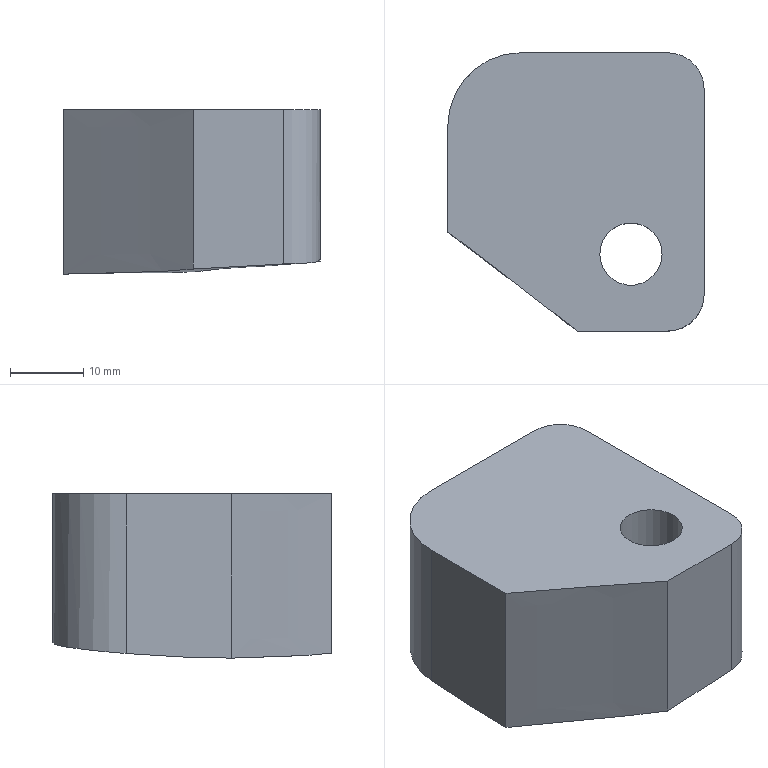Part | STEP file | gslz 2016.10.28-10_id1662_x_t | 1 solid | 13 faces | volume 22652 mm3 | plane 6 | cylinder 5 | spline 1 | other 1 | commonest cylinder face diameters 10 x2 8.5 x1 14 x1 20 x1